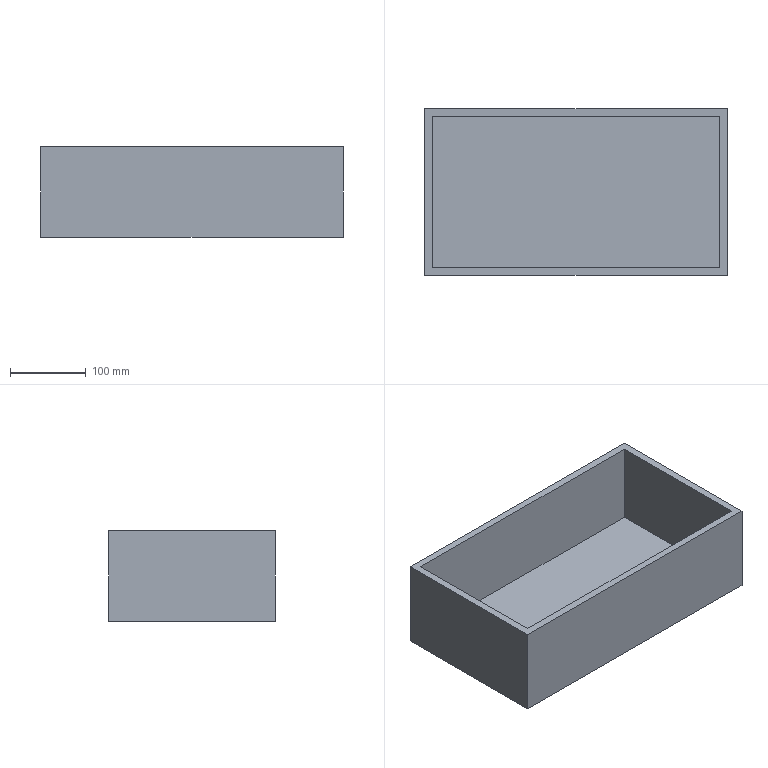Part | SolidWorks | features ExtruThin 1, ICE 1 | 1 solid | 11 faces | box 400 x 220 x 120 mm | volume 2200000 mm3 | plane 11
STEP:
#1=CARTESIAN_POINT('',(190.,100.,120.));
#2=VERTEX_POINT('',#1);
#3=CARTESIAN_POINT('',(190.,100.,10.));
#4=VERTEX_POINT('',#3);
#5=CARTESIAN_POINT('',(190.,100.,120.));
#6=DIRECTION('',(0.,0.,-1.));
#7=VECTOR('',#6,1000.);
#8=LINE('',#5,#7);
#9=EDGE_CURVE('',#2,#4,#8,.T.);
#10=ORIENTED_EDGE('',*,*,#9,.T.);
#11=CARTESIAN_POINT('',(190.,-100.,10.));
#12=VERTEX_POINT('',#11);
#13=CARTESIAN_POINT('',(190.,-100.,10.));
#14=DIRECTION('',(0.,-1.,0.));
#15=VECTOR('',#14,1000.);
#16=LINE('',#13,#15);
#17=EDGE_CURVE('',#4,#12,#16,.T.);
#18=ORIENTED_EDGE('',*,*,#17,.T.);
#19=CARTESIAN_POINT('',(190.,-100.,120.));
#20=VERTEX_POINT('',#19);
#21=CARTESIAN_POINT('',(190.,-100.,120.));
#22=DIRECTION('',(0.,0.,-1.));
#23=VECTOR('',#22,1000.);
#24=LINE('',#21,#23);
#25=EDGE_CURVE('',#20,#12,#24,.T.);
#26=ORIENTED_EDGE('',*,*,#25,.F.);
#27=CARTESIAN_POINT('',(190.,-100.,120.));
#28=DIRECTION('',(0.,1.,0.));
#29=VECTOR('',#28,1000.);
#30=LINE('',#27,#29);
#31=EDGE_CURVE('',#20,#2,#30,.T.);
#32=ORIENTED_EDGE('',*,*,#31,.T.);
#33=EDGE_LOOP('',(#10,#18,#26,#32));
#34=FACE_OUTER_BOUND('',#33,.T.);
#35=CARTESIAN_POINT('',(190.,-100.,120.));
#36=DIRECTION('',(-1.,0.,0.));
#37=DIRECTION('',(0.,0.,1.));
#38=AXIS2_PLACEMENT_3D('',#35,#36,#37);
#39=PLANE('',#38);
#40=ADVANCED_FACE('',(#34),#39,.T.);
#41=CARTESIAN_POINT('',(-190.,100.,120.));
#42=VERTEX_POINT('',#41);
#43=CARTESIAN_POINT('',(-190.,100.,10.));
#44=VERTEX_POINT('',#43);
#45=CARTESIAN_POINT('',(-190.,100.,120.));
#46=DIRECTION('',(0.,0.,-1.));
#47=VECTOR('',#46,1000.);
#48=LINE('',#45,#47);
#49=EDGE_CURVE('',#42,#44,#48,.T.);
#50=ORIENTED_EDGE('',*,*,#49,.T.);
#51=CARTESIAN_POINT('',(-200.,100.,10.));
#52=DIRECTION('',(-1.,0.,0.));
#53=VECTOR('',#52,1000.);
#54=LINE('',#51,#53);
#55=EDGE_CURVE('',#4,#44,#54,.T.);
#56=ORIENTED_EDGE('',*,*,#55,.F.);
#57=ORIENTED_EDGE('',*,*,#9,.F.);
#58=CARTESIAN_POINT('',(-190.,100.,120.));
#59=DIRECTION('',(-1.,0.,0.));
#60=VECTOR('',#59,1000.);
#61=LINE('',#58,#60);
#62=EDGE_CURVE('',#2,#42,#61,.T.);
#63=ORIENTED_EDGE('',*,*,#62,.T.);
#64=EDGE_LOOP('',(#50,#56,#57,#63));
#65=FACE_OUTER_BOUND('',#64,.T.);
#66=CARTESIAN_POINT('',(-190.,100.,120.));
#67=DIRECTION('',(0.,-1.,0.));
#68=DIRECTION('',(0.,0.,-1.));
#69=AXIS2_PLACEMENT_3D('',#66,#67,#68);
#70=PLANE('',#69);
#71=ADVANCED_FACE('',(#65),#70,.T.);
#72=CARTESIAN_POINT('',(-190.,-100.,120.));
#73=VERTEX_POINT('',#72);
#74=CARTESIAN_POINT('',(-190.,-100.,10.));
#75=VERTEX_POINT('',#74);
#76=CARTESIAN_POINT('',(-190.,-100.,120.));
#77=DIRECTION('',(0.,0.,-1.));
#78=VECTOR('',#77,1000.);
#79=LINE('',#76,#78);
#80=EDGE_CURVE('',#73,#75,#79,.T.);
#81=ORIENTED_EDGE('',*,*,#80,.T.);
#82=CARTESIAN_POINT('',(-190.,-100.,10.));
#83=DIRECTION('',(0.,1.,0.));
#84=VECTOR('',#83,1000.);
#85=LINE('',#82,#84);
#86=EDGE_CURVE('',#75,#44,#85,.T.);
#87=ORIENTED_EDGE('',*,*,#86,.T.);
#88=ORIENTED_EDGE('',*,*,#49,.F.);
#89=CARTESIAN_POINT('',(-190.,-100.,120.));
#90=DIRECTION('',(0.,-1.,0.));
#91=VECTOR('',#90,1000.);
#92=LINE('',#89,#91);
#93=EDGE_CURVE('',#42,#73,#92,.T.);
#94=ORIENTED_EDGE('',*,*,#93,.T.);
#95=EDGE_LOOP('',(#81,#87,#88,#94));
#96=FACE_OUTER_BOUND('',#95,.T.);
#97=CARTESIAN_POINT('',(-190.,-100.,120.));
#98=DIRECTION('',(1.,0.,0.));
#99=DIRECTION('',(0.,0.,-1.));
#100=AXIS2_PLACEMENT_3D('',#97,#98,#99);
#101=PLANE('',#100);
#102=ADVANCED_FACE('',(#96),#101,.T.);
#103=ORIENTED_EDGE('',*,*,#25,.T.);
#104=CARTESIAN_POINT('',(-190.,-100.,10.));
#105=DIRECTION('',(-1.,0.,0.));
#106=VECTOR('',#105,1000.);
#107=LINE('',#104,#106);
#108=EDGE_CURVE('',#12,#75,#107,.T.);
#109=ORIENTED_EDGE('',*,*,#108,.T.);
#110=ORIENTED_EDGE('',*,*,#80,.F.);
#111=CARTESIAN_POINT('',(-190.,-100.,120.));
#112=DIRECTION('',(1.,0.,0.));
#113=VECTOR('',#112,1000.);
#114=LINE('',#111,#113);
#115=EDGE_CURVE('',#73,#20,#114,.T.);
#116=ORIENTED_EDGE('',*,*,#115,.T.);
#117=EDGE_LOOP('',(#103,#109,#110,#116));
#118=FACE_OUTER_BOUND('',#117,.T.);
#119=CARTESIAN_POINT('',(-190.,-100.,120.));
#120=DIRECTION('',(0.,1.,0.));
#121=DIRECTION('',(0.,0.,1.));
#122=AXIS2_PLACEMENT_3D('',#119,#120,#121);
#123=PLANE('',#122);
#124=ADVANCED_FACE('',(#118),#123,.T.);
#125=CARTESIAN_POINT('',(200.,-110.,120.));
#126=VERTEX_POINT('',#125);
#127=CARTESIAN_POINT('',(200.,110.,120.));
#128=VERTEX_POINT('',#127);
#129=CARTESIAN_POINT('',(200.,0.,120.));
#130=DIRECTION('',(0.,1.,0.));
#131=VECTOR('',#130,1000.);
#132=LINE('',#129,#131);
#133=EDGE_CURVE('',#126,#128,#132,.T.);
#134=ORIENTED_EDGE('',*,*,#133,.T.);
#135=CARTESIAN_POINT('',(-200.,110.,120.));
#136=VERTEX_POINT('',#135);
#137=CARTESIAN_POINT('',(0.,110.,120.));
#138=DIRECTION('',(-1.,0.,0.));
#139=VECTOR('',#138,1000.);
#140=LINE('',#137,#139);
#141=EDGE_CURVE('',#128,#136,#140,.T.);
#142=ORIENTED_EDGE('',*,*,#141,.T.);
#143=CARTESIAN_POINT('',(-200.,-110.,120.));
#144=VERTEX_POINT('',#143);
#145=CARTESIAN_POINT('',(-200.,0.,120.));
#146=DIRECTION('',(0.,-1.,0.));
#147=VECTOR('',#146,1000.);
#148=LINE('',#145,#147);
#149=EDGE_CURVE('',#136,#144,#148,.T.);
#150=ORIENTED_EDGE('',*,*,#149,.T.);
#151=CARTESIAN_POINT('',(0.,-110.,120.));
#152=DIRECTION('',(1.,0.,0.));
#153=VECTOR('',#152,1000.);
#154=LINE('',#151,#153);
#155=EDGE_CURVE('',#144,#126,#154,.T.);
#156=ORIENTED_EDGE('',*,*,#155,.T.);
#157=EDGE_LOOP('',(#134,#142,#150,#156));
#158=FACE_OUTER_BOUND('',#157,.T.);
#159=ORIENTED_EDGE('',*,*,#62,.F.);
#160=ORIENTED_EDGE('',*,*,#31,.F.);
#161=ORIENTED_EDGE('',*,*,#115,.F.);
#162=ORIENTED_EDGE('',*,*,#93,.F.);
#163=EDGE_LOOP('',(#159,#160,#161,#162));
#164=FACE_BOUND('',#163,.T.);
#165=CARTESIAN_POINT('',(0.,0.,120.));
#166=DIRECTION('',(0.,0.,1.));
#167=DIRECTION('',(1.,0.,0.));
#168=AXIS2_PLACEMENT_3D('',#165,#166,#167);
#169=PLANE('',#168);
#170=ADVANCED_FACE('',(#158,#164),#169,.T.);
#171=CARTESIAN_POINT('',(-200.,-110.,0.));
#172=VERTEX_POINT('',#171);
#173=CARTESIAN_POINT('',(200.,-110.,0.));
#174=VERTEX_POINT('',#173);
#175=CARTESIAN_POINT('',(0.,-110.,0.));
#176=DIRECTION('',(1.,0.,0.));
#177=VECTOR('',#176,1000.);
#178=LINE('',#175,#177);
#179=EDGE_CURVE('',#172,#174,#178,.T.);
#180=ORIENTED_EDGE('',*,*,#179,.F.);
#181=CARTESIAN_POINT('',(-200.,110.,0.));
#182=VERTEX_POINT('',#181);
#183=CARTESIAN_POINT('',(-200.,0.,0.));
#184=DIRECTION('',(0.,-1.,0.));
#185=VECTOR('',#184,1000.);
#186=LINE('',#183,#185);
#187=EDGE_CURVE('',#182,#172,#186,.T.);
#188=ORIENTED_EDGE('',*,*,#187,.F.);
#189=CARTESIAN_POINT('',(200.,110.,0.));
#190=VERTEX_POINT('',#189);
#191=CARTESIAN_POINT('',(0.,110.,0.));
#192=DIRECTION('',(-1.,0.,0.));
#193=VECTOR('',#192,1000.);
#194=LINE('',#191,#193);
#195=EDGE_CURVE('',#190,#182,#194,.T.);
#196=ORIENTED_EDGE('',*,*,#195,.F.);
#197=CARTESIAN_POINT('',(200.,0.,0.));
#198=DIRECTION('',(0.,1.,0.));
#199=VECTOR('',#198,1000.);
#200=LINE('',#197,#199);
#201=EDGE_CURVE('',#174,#190,#200,.T.);
#202=ORIENTED_EDGE('',*,*,#201,.F.);
#203=EDGE_LOOP('',(#180,#188,#196,#202));
#204=FACE_OUTER_BOUND('',#203,.T.);
#205=CARTESIAN_POINT('',(0.,0.,0.));
#206=DIRECTION('',(0.,0.,1.));
#207=DIRECTION('',(1.,0.,0.));
#208=AXIS2_PLACEMENT_3D('',#205,#206,#207);
#209=PLANE('',#208);
#210=ADVANCED_FACE('',(#204),#209,.F.);
#211=ORIENTED_EDGE('',*,*,#201,.T.);
#212=CARTESIAN_POINT('',(200.,110.,120.));
#213=DIRECTION('',(0.,0.,-1.));
#214=VECTOR('',#213,1000.);
#215=LINE('',#212,#214);
#216=EDGE_CURVE('',#128,#190,#215,.T.);
#217=ORIENTED_EDGE('',*,*,#216,.F.);
#218=ORIENTED_EDGE('',*,*,#133,.F.);
#219=CARTESIAN_POINT('',(200.,-110.,120.));
#220=DIRECTION('',(0.,0.,-1.));
#221=VECTOR('',#220,1000.);
#222=LINE('',#219,#221);
#223=EDGE_CURVE('',#126,#174,#222,.T.);
#224=ORIENTED_EDGE('',*,*,#223,.T.);
#225=EDGE_LOOP('',(#211,#217,#218,#224));
#226=FACE_OUTER_BOUND('',#225,.T.);
#227=CARTESIAN_POINT('',(200.,0.,120.));
#228=DIRECTION('',(-1.,0.,0.));
#229=DIRECTION('',(0.,0.,1.));
#230=AXIS2_PLACEMENT_3D('',#227,#228,#229);
#231=PLANE('',#230);
#232=ADVANCED_FACE('',(#226),#231,.F.);
#233=ORIENTED_EDGE('',*,*,#195,.T.);
#234=CARTESIAN_POINT('',(-200.,110.,120.));
#235=DIRECTION('',(0.,0.,-1.));
#236=VECTOR('',#235,1000.);
#237=LINE('',#234,#236);
#238=EDGE_CURVE('',#136,#182,#237,.T.);
#239=ORIENTED_EDGE('',*,*,#238,.F.);
#240=ORIENTED_EDGE('',*,*,#141,.F.);
#241=ORIENTED_EDGE('',*,*,#216,.T.);
#242=EDGE_LOOP('',(#233,#239,#240,#241));
#243=FACE_OUTER_BOUND('',#242,.T.);
#244=CARTESIAN_POINT('',(0.,110.,120.));
#245=DIRECTION('',(0.,-1.,0.));
#246=DIRECTION('',(0.,0.,-1.));
#247=AXIS2_PLACEMENT_3D('',#244,#245,#246);
#248=PLANE('',#247);
#249=ADVANCED_FACE('',(#243),#248,.F.);
#250=ORIENTED_EDGE('',*,*,#187,.T.);
#251=CARTESIAN_POINT('',(-200.,-110.,120.));
#252=DIRECTION('',(0.,0.,-1.));
#253=VECTOR('',#252,1000.);
#254=LINE('',#251,#253);
#255=EDGE_CURVE('',#144,#172,#254,.T.);
#256=ORIENTED_EDGE('',*,*,#255,.F.);
#257=ORIENTED_EDGE('',*,*,#149,.F.);
#258=ORIENTED_EDGE('',*,*,#238,.T.);
#259=EDGE_LOOP('',(#250,#256,#257,#258));
#260=FACE_OUTER_BOUND('',#259,.T.);
#261=CARTESIAN_POINT('',(-200.,0.,120.));
#262=DIRECTION('',(1.,0.,0.));
#263=DIRECTION('',(0.,0.,-1.));
#264=AXIS2_PLACEMENT_3D('',#261,#262,#263);
#265=PLANE('',#264);
#266=ADVANCED_FACE('',(#260),#265,.F.);
#267=ORIENTED_EDGE('',*,*,#179,.T.);
#268=ORIENTED_EDGE('',*,*,#223,.F.);
#269=ORIENTED_EDGE('',*,*,#155,.F.);
#270=ORIENTED_EDGE('',*,*,#255,.T.);
#271=EDGE_LOOP('',(#267,#268,#269,#270));
#272=FACE_OUTER_BOUND('',#271,.T.);
#273=CARTESIAN_POINT('',(0.,-110.,120.));
#274=DIRECTION('',(0.,1.,0.));
#275=DIRECTION('',(0.,0.,1.));
#276=AXIS2_PLACEMENT_3D('',#273,#274,#275);
#277=PLANE('',#276);
#278=ADVANCED_FACE('',(#272),#277,.F.);
#279=ORIENTED_EDGE('',*,*,#17,.F.);
#280=ORIENTED_EDGE('',*,*,#55,.T.);
#281=ORIENTED_EDGE('',*,*,#86,.F.);
#282=ORIENTED_EDGE('',*,*,#108,.F.);
#283=EDGE_LOOP('',(#279,#280,#281,#282));
#284=FACE_OUTER_BOUND('',#283,.T.);
#285=CARTESIAN_POINT('',(-200.,-510.125,10.));
#286=DIRECTION('',(0.,0.,-1.));
#287=DIRECTION('',(-1.,0.,0.));
#288=AXIS2_PLACEMENT_3D('',#285,#286,#287);
#289=PLANE('',#288);
#290=ADVANCED_FACE('',(#284),#289,.F.);
#291=CLOSED_SHELL('',(#40,#71,#102,#124,#170,#210,#232,#249,#266,#278,#290));
#292=MANIFOLD_SOLID_BREP('',#291);
#293=CARTESIAN_POINT('',(0.,0.,0.));
#294=DIRECTION('',(0.,0.,1.));
#295=DIRECTION('',(1.,0.,0.));
#296=AXIS2_PLACEMENT_3D('',#293,#294,#295);
#297=(LENGTH_UNIT()NAMED_UNIT(*)SI_UNIT(.MILLI.,.METRE.));
#298=UNCERTAINTY_MEASURE_WITH_UNIT(LENGTH_MEASURE(0.00001),#297,'','');
#299=(NAMED_UNIT(*)PLANE_ANGLE_UNIT()SI_UNIT($,.RADIAN.));
#300=(NAMED_UNIT(*)SI_UNIT($,.STERADIAN.)SOLID_ANGLE_UNIT());
#301=(GEOMETRIC_REPRESENTATION_CONTEXT(3)GLOBAL_UNCERTAINTY_ASSIGNED_CONTEXT((#298))GLOBAL_UNIT_ASSIGNED_CONTEXT((#297,#299,#300))REPRESENTATION_CONTEXT('',''));
#302=ADVANCED_BREP_SHAPE_REPRESENTATION('',(#292,#296),#301);